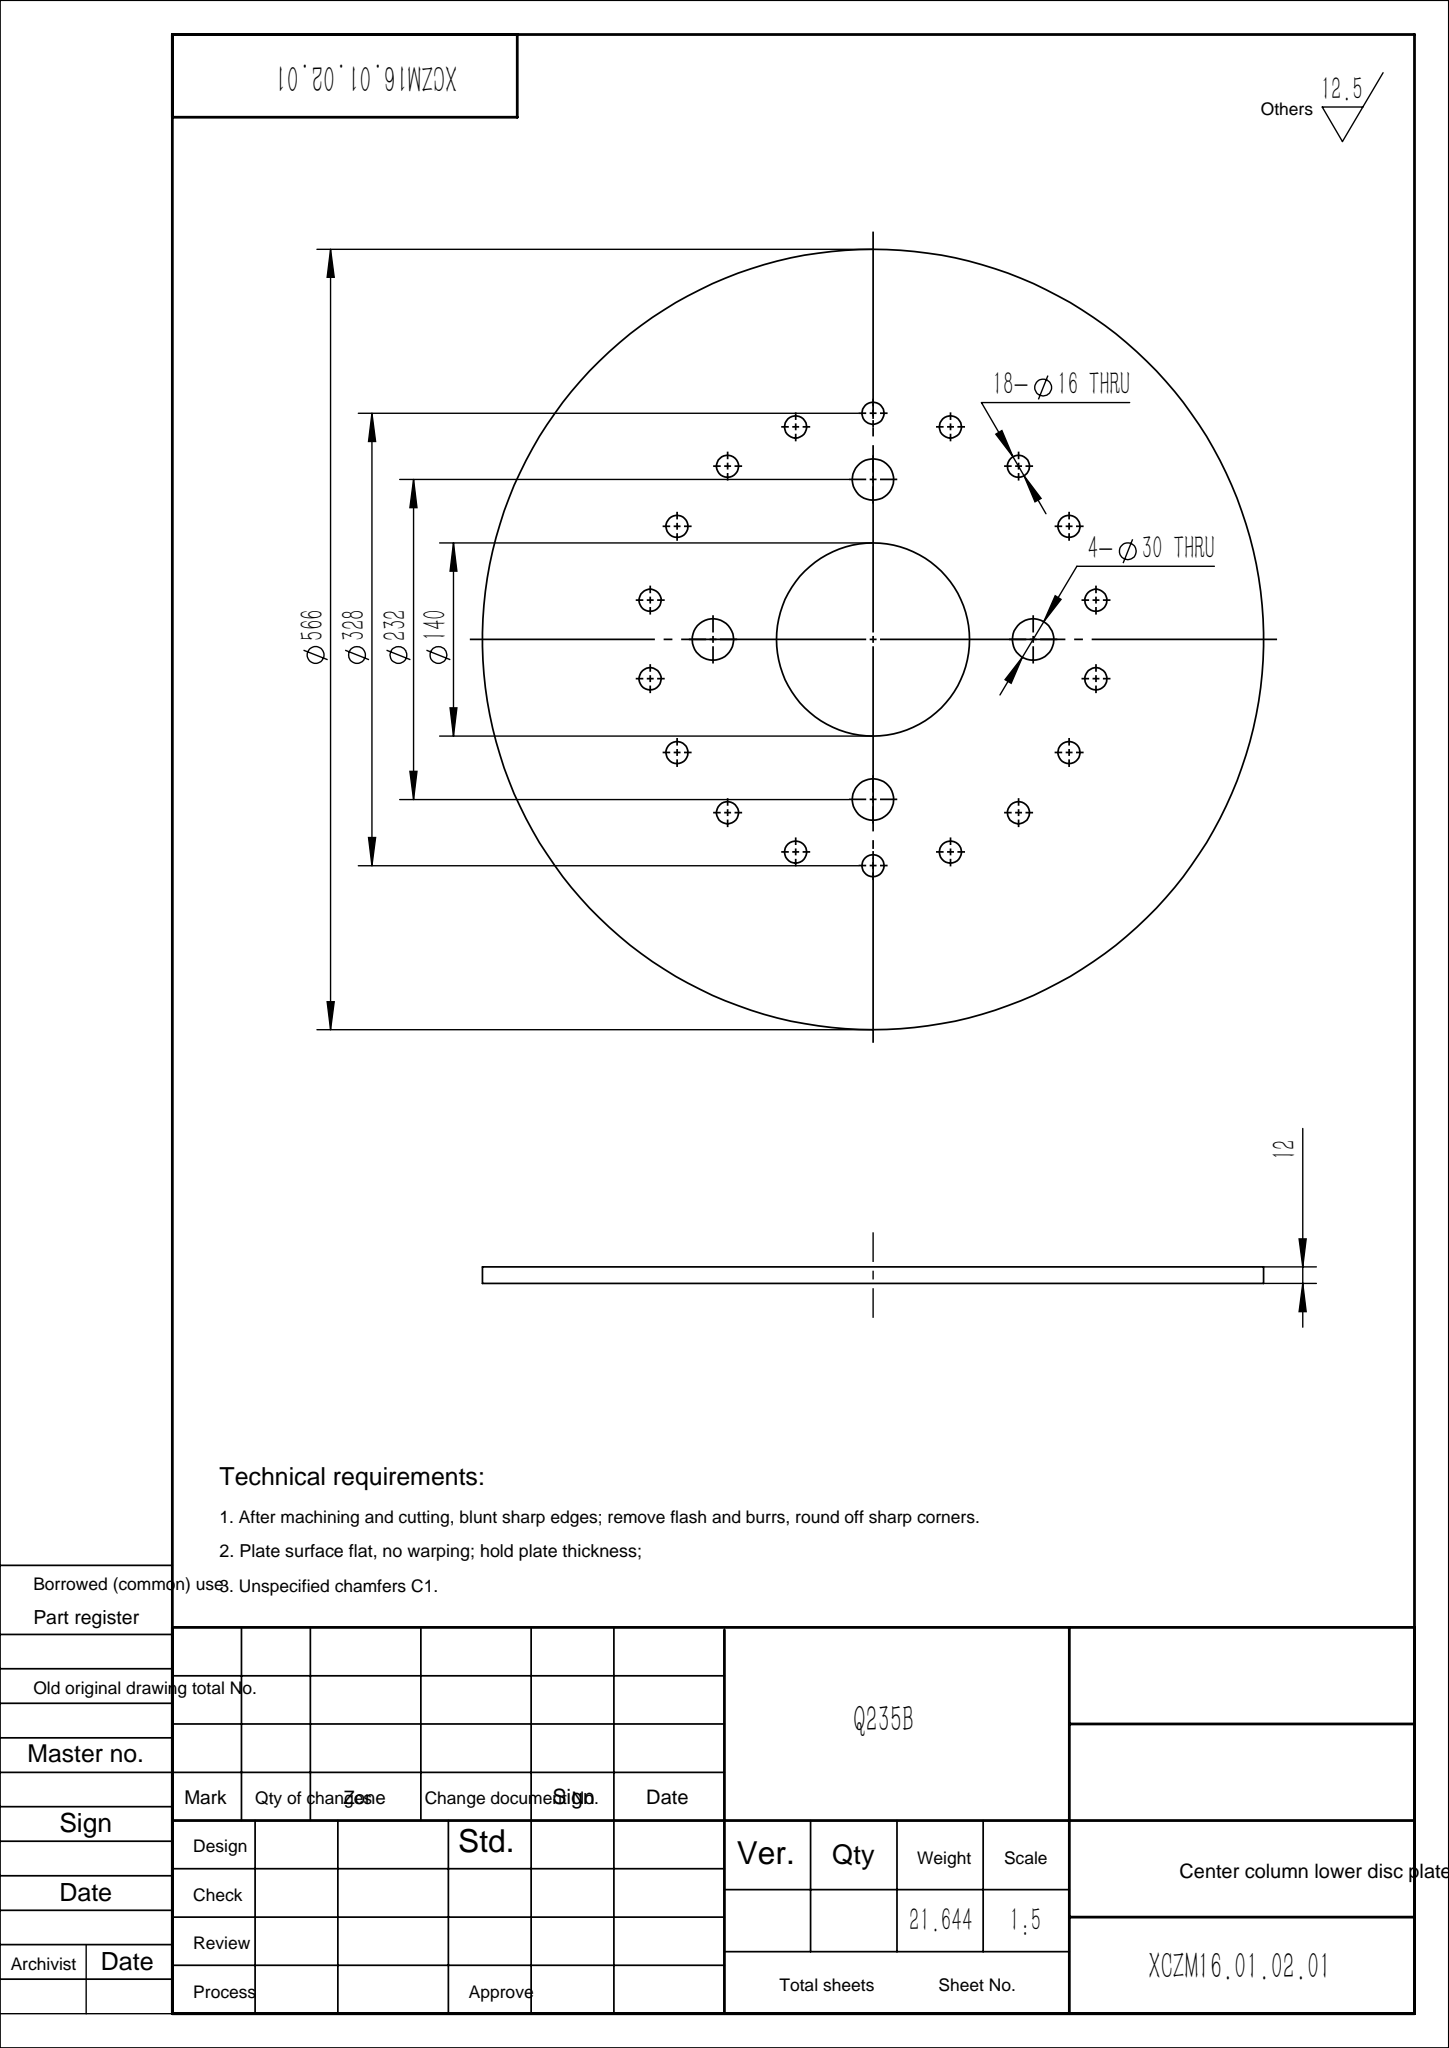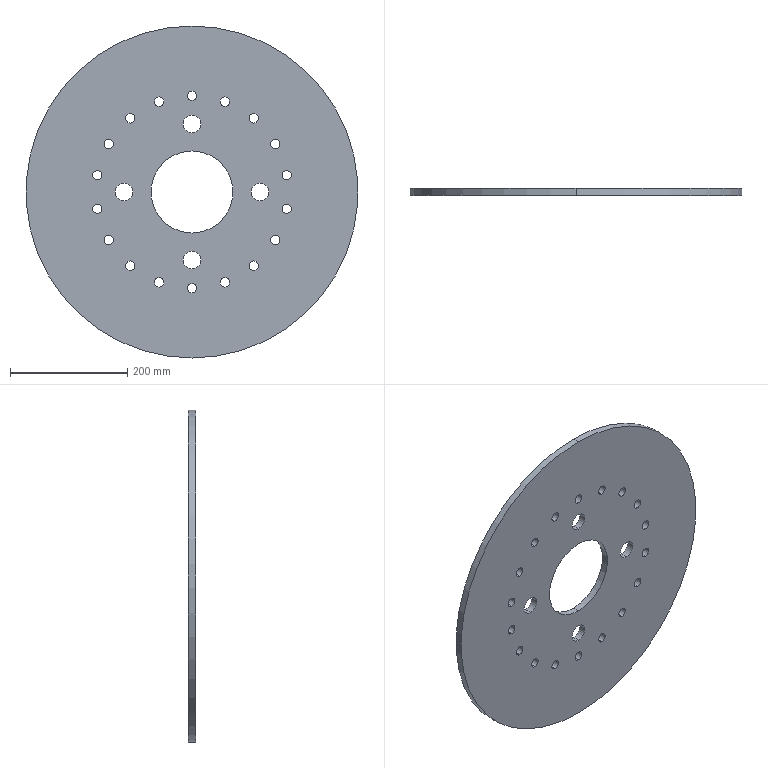Part | SolidWorks | features Extrusion 1 | 1 solid | 50 faces | box 566 x 12 x 566 mm | volume 2757200 mm3 | cylinder 48 | plane 2 | commonest cylinder face diameters 16 x36 30 x8 140 x2 566 x2